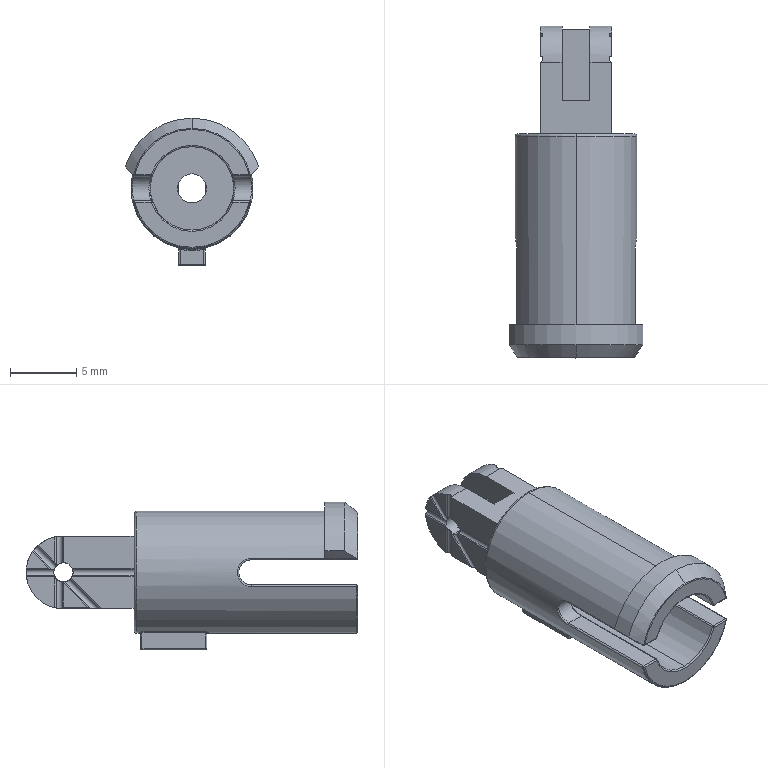Part | SolidWorks | features ICE 8, Fillet 3, MirrorPattern 1, Revolution 1 | 1 solid | 145 faces | box 10.095 x 25.05 x 11.15 mm | volume 779.469 mm3 | cylinder 75 | plane 40 | torus 11 | sphere 8 | spline 8 | cone 3 | commonest cylinder face diameters 0.2 x47 0.51 x8 0.513 x6 1.45 x4 1.9 x2 2.2 x2